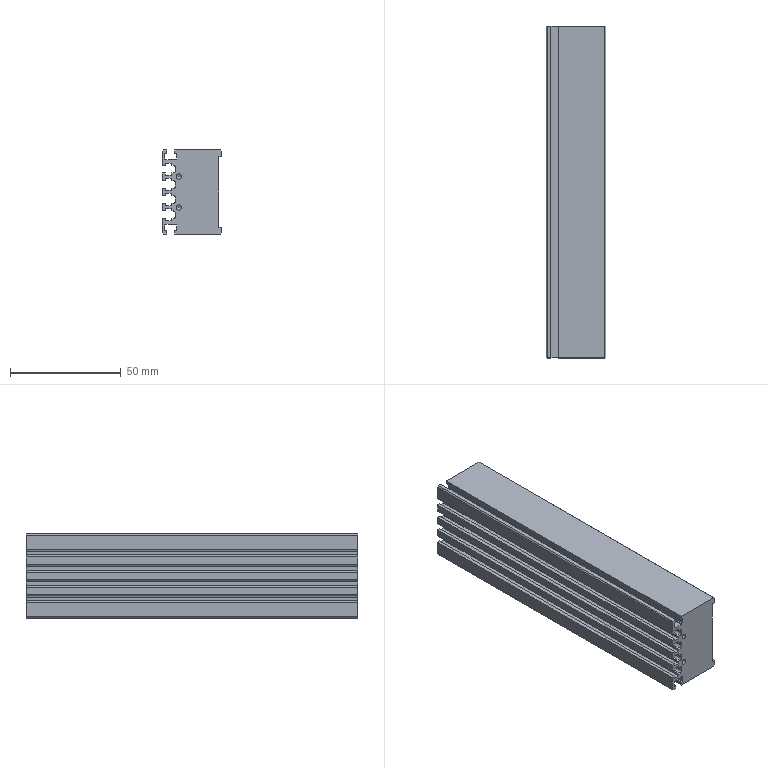Part | STEP file | CST-2BS14738W-1-1-11111 | 1 solid | 102 faces | box 27.023 x 150 x 38 mm | volume 125802 mm3 | plane 86 | cylinder 12 | cone 4 | commonest cylinder face diameters 2 x8 2.46 x4